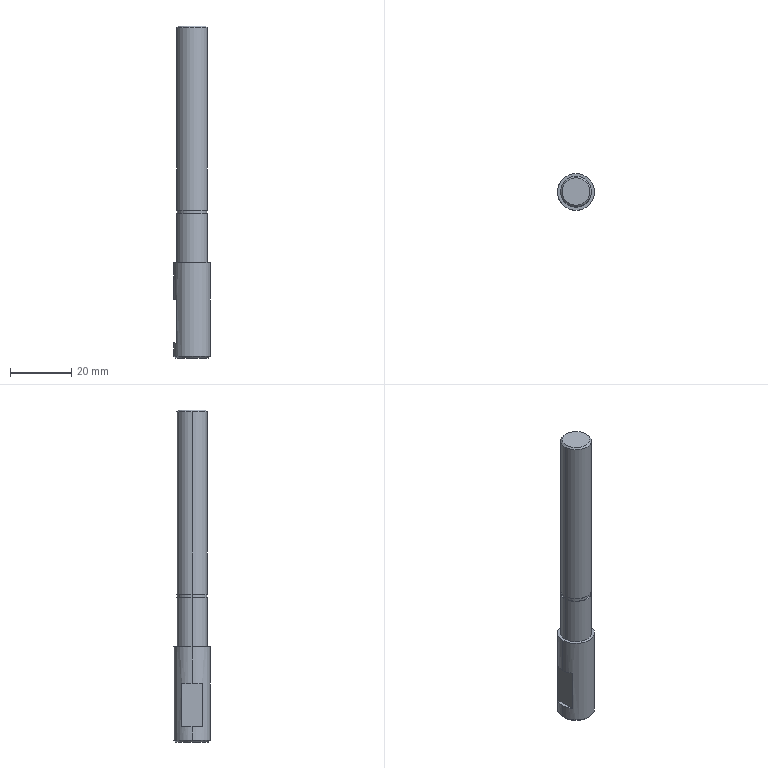Part | STEP file | PN_0097 linear shaft | 1 solid | 20 faces | box 12 x 12 x 108 mm | volume 9475 mm3 | cylinder 8 | plane 8 | cone 4 | commonest cylinder face diameters 10 x4 9.6 x2 12 x2
STEP:
#1=CARTESIAN_POINT('',(0.,0.,0.));
#2=DIRECTION('',(0.,0.,1.));
#3=DIRECTION('',(1.,0.,0.));
#4=AXIS2_PLACEMENT_3D('',#1,#2,#3);
#5=CARTESIAN_POINT('',(-5.5,0.,0.));
#6=VERTEX_POINT('',#5);
#7=CARTESIAN_POINT('',(5.5,0.,0.));
#8=VERTEX_POINT('',#7);
#9=CARTESIAN_POINT('',(0.,0.,0.));
#10=DIRECTION('',(0.,0.,-1.));
#11=DIRECTION('',(1.,0.,0.));
#12=AXIS2_PLACEMENT_3D('',#9,#10,#11);
#13=CIRCLE('',#12,5.5);
#14=CARTESIAN_POINT('',(0.,0.,0.5));
#15=DIRECTION('',(0.,0.,1.));
#16=DIRECTION('',(1.,0.,0.));
#17=AXIS2_PLACEMENT_3D('',#14,#15,#16);
#18=CONICAL_SURFACE('',#17,6.,0.7854);
#19=CARTESIAN_POINT('',(6.283,-0.5));
#20=DIRECTION('',(-1.,0.));
#21=VECTOR('',#20,1.);
#22=LINE('',#19,#21);
#23=(GEOMETRIC_REPRESENTATION_CONTEXT(2)PARAMETRIC_REPRESENTATION_CONTEXT()REPRESENTATION_CONTEXT('',''));
#24=DEFINITIONAL_REPRESENTATION('',(#22),#23);
#25=PCURVE('',#18,#24);
#26=CARTESIAN_POINT('',(0.,0.,0.));
#27=DIRECTION('',(0.,0.,1.));
#28=DIRECTION('',(1.,0.,0.));
#29=AXIS2_PLACEMENT_3D('',#26,#27,#28);
#30=PLANE('',#29);
#31=CARTESIAN_POINT('',(5.5,0.));
#32=CARTESIAN_POINT('',(5.5,-9.526));
#33=CARTESIAN_POINT('',(-2.75,-4.763));
#34=CARTESIAN_POINT('',(-11.,0.));
#35=CARTESIAN_POINT('',(-2.75,4.763));
#36=CARTESIAN_POINT('',(5.5,9.526));
#37=CARTESIAN_POINT('',(5.5,0.));
#38=(BOUNDED_CURVE()B_SPLINE_CURVE(2,(#31,#32,#33,#34,#35,#36,#37),.UNSPECIFIED.,.T.,.F.)B_SPLINE_CURVE_WITH_KNOTS((1,2,2,2,2,1),(-2.094,0.,2.094,4.189,6.283,8.378),.UNSPECIFIED.)CURVE()GEOMETRIC_REPRESENTATION_ITEM()RATIONAL_B_SPLINE_CURVE((1.,0.5,1.,0.5,1.,0.5,1.))REPRESENTATION_ITEM(''));
#39=(GEOMETRIC_REPRESENTATION_CONTEXT(2)PARAMETRIC_REPRESENTATION_CONTEXT()REPRESENTATION_CONTEXT('',''));
#40=DEFINITIONAL_REPRESENTATION('',(#38),#39);
#41=PCURVE('',#30,#40);
#42=SURFACE_CURVE('',#13,(#25,#41),.PCURVE_S1.);
#43=EDGE_CURVE('',#6,#8,#42,.T.);
#44=ORIENTED_EDGE('',*,*,#43,.F.);
#45=CARTESIAN_POINT('',(-6.,0.,0.5));
#46=VERTEX_POINT('',#45);
#47=CARTESIAN_POINT('',(-6.,0.,0.5));
#48=DIRECTION('',(-0.7071,0.,0.7071));
#49=VECTOR('',#48,1.);
#50=LINE('',#47,#49);
#51=CARTESIAN_POINT('',(3.142,0.));
#52=DIRECTION('',(0.,1.));
#53=VECTOR('',#52,1.);
#54=LINE('',#51,#53);
#55=(GEOMETRIC_REPRESENTATION_CONTEXT(2)PARAMETRIC_REPRESENTATION_CONTEXT()REPRESENTATION_CONTEXT('',''));
#56=DEFINITIONAL_REPRESENTATION('',(#54),#55);
#57=PCURVE('',#18,#56);
#58=CARTESIAN_POINT('',(0.,0.,0.5));
#59=DIRECTION('',(0.,0.,1.));
#60=DIRECTION('',(1.,0.,0.));
#61=AXIS2_PLACEMENT_3D('',#58,#59,#60);
#62=CONICAL_SURFACE('',#61,6.,0.7854);
#63=CARTESIAN_POINT('',(3.142,0.));
#64=DIRECTION('',(0.,1.));
#65=VECTOR('',#64,1.);
#66=LINE('',#63,#65);
#67=(GEOMETRIC_REPRESENTATION_CONTEXT(2)PARAMETRIC_REPRESENTATION_CONTEXT()REPRESENTATION_CONTEXT('',''));
#68=DEFINITIONAL_REPRESENTATION('',(#66),#67);
#69=PCURVE('',#62,#68);
#70=SURFACE_CURVE('',#50,(#57,#69),.PCURVE_S1.);
#71=EDGE_CURVE('',#6,#46,#70,.T.);
#72=ORIENTED_EDGE('',*,*,#71,.T.);
#73=CARTESIAN_POINT('',(6.,0.,0.5));
#74=VERTEX_POINT('',#73);
#75=CARTESIAN_POINT('',(0.,0.,0.5));
#76=DIRECTION('',(0.,0.,1.));
#77=DIRECTION('',(1.,0.,0.));
#78=AXIS2_PLACEMENT_3D('',#75,#76,#77);
#79=CIRCLE('',#78,6.);
#80=CARTESIAN_POINT('',(0.,0.));
#81=DIRECTION('',(1.,0.));
#82=VECTOR('',#81,1.);
#83=LINE('',#80,#82);
#84=(GEOMETRIC_REPRESENTATION_CONTEXT(2)PARAMETRIC_REPRESENTATION_CONTEXT()REPRESENTATION_CONTEXT('',''));
#85=DEFINITIONAL_REPRESENTATION('',(#83),#84);
#86=PCURVE('',#18,#85);
#87=CARTESIAN_POINT('',(0.,0.,31.));
#88=DIRECTION('',(0.,0.,-1.));
#89=DIRECTION('',(-1.,0.,0.));
#90=AXIS2_PLACEMENT_3D('',#87,#88,#89);
#91=CYLINDRICAL_SURFACE('',#90,6.);
#92=CARTESIAN_POINT('',(3.142,30.5));
#93=DIRECTION('',(-1.,0.));
#94=VECTOR('',#93,1.);
#95=LINE('',#92,#94);
#96=(GEOMETRIC_REPRESENTATION_CONTEXT(2)PARAMETRIC_REPRESENTATION_CONTEXT()REPRESENTATION_CONTEXT('',''));
#97=DEFINITIONAL_REPRESENTATION('',(#95),#96);
#98=PCURVE('',#91,#97);
#99=SURFACE_CURVE('',#79,(#86,#98),.PCURVE_S1.);
#100=EDGE_CURVE('',#74,#46,#99,.T.);
#101=ORIENTED_EDGE('',*,*,#100,.F.);
#102=CARTESIAN_POINT('',(6.,0.,0.5));
#103=DIRECTION('',(0.7071,0.,0.7071));
#104=VECTOR('',#103,1.);
#105=LINE('',#102,#104);
#106=CARTESIAN_POINT('',(0.,0.));
#107=DIRECTION('',(0.,1.));
#108=VECTOR('',#107,1.);
#109=LINE('',#106,#108);
#110=(GEOMETRIC_REPRESENTATION_CONTEXT(2)PARAMETRIC_REPRESENTATION_CONTEXT()REPRESENTATION_CONTEXT('',''));
#111=DEFINITIONAL_REPRESENTATION('',(#109),#110);
#112=PCURVE('',#18,#111);
#113=CARTESIAN_POINT('',(6.283,0.));
#114=DIRECTION('',(0.,1.));
#115=VECTOR('',#114,1.);
#116=LINE('',#113,#115);
#117=(GEOMETRIC_REPRESENTATION_CONTEXT(2)PARAMETRIC_REPRESENTATION_CONTEXT()REPRESENTATION_CONTEXT('',''));
#118=DEFINITIONAL_REPRESENTATION('',(#116),#117);
#119=PCURVE('',#62,#118);
#120=SURFACE_CURVE('',#105,(#112,#119),.PCURVE_S1.);
#121=EDGE_CURVE('',#8,#74,#120,.T.);
#122=ORIENTED_EDGE('',*,*,#121,.F.);
#123=EDGE_LOOP('',(#44,#72,#101,#122));
#124=FACE_BOUND('',#123,.T.);
#125=ADVANCED_FACE('',(#124),#18,.T.);
#126=CARTESIAN_POINT('',(4.5,0.,108.));
#127=VERTEX_POINT('',#126);
#128=CARTESIAN_POINT('',(-4.5,0.,108.));
#129=VERTEX_POINT('',#128);
#130=CARTESIAN_POINT('',(0.,0.,108.));
#131=DIRECTION('',(0.,0.,1.));
#132=DIRECTION('',(1.,0.,0.));
#133=AXIS2_PLACEMENT_3D('',#130,#131,#132);
#134=CIRCLE('',#133,4.5);
#135=CARTESIAN_POINT('',(0.,0.,108.));
#136=DIRECTION('',(0.,0.,-1.));
#137=DIRECTION('',(-1.,0.,0.));
#138=AXIS2_PLACEMENT_3D('',#135,#136,#137);
#139=CONICAL_SURFACE('',#138,4.5,0.7854);
#140=CARTESIAN_POINT('',(3.142,0.));
#141=DIRECTION('',(-1.,0.));
#142=VECTOR('',#141,1.);
#143=LINE('',#140,#142);
#144=(GEOMETRIC_REPRESENTATION_CONTEXT(2)PARAMETRIC_REPRESENTATION_CONTEXT()REPRESENTATION_CONTEXT('',''));
#145=DEFINITIONAL_REPRESENTATION('',(#143),#144);
#146=PCURVE('',#139,#145);
#147=CARTESIAN_POINT('',(0.,0.,108.));
#148=DIRECTION('',(0.,0.,1.));
#149=DIRECTION('',(1.,0.,0.));
#150=AXIS2_PLACEMENT_3D('',#147,#148,#149);
#151=PLANE('',#150);
#152=CARTESIAN_POINT('',(0.,0.));
#153=DIRECTION('',(1.,0.));
#154=AXIS2_PLACEMENT_2D('',#152,#153);
#155=CIRCLE('',#154,4.5);
#156=(GEOMETRIC_REPRESENTATION_CONTEXT(2)PARAMETRIC_REPRESENTATION_CONTEXT()REPRESENTATION_CONTEXT('',''));
#157=DEFINITIONAL_REPRESENTATION('',(#155),#156);
#158=PCURVE('',#151,#157);
#159=SURFACE_CURVE('',#134,(#146,#158),.PCURVE_S1.);
#160=EDGE_CURVE('',#127,#129,#159,.T.);
#161=ORIENTED_EDGE('',*,*,#160,.F.);
#162=CARTESIAN_POINT('',(5.,0.,107.5));
#163=VERTEX_POINT('',#162);
#164=CARTESIAN_POINT('',(4.5,0.,108.));
#165=DIRECTION('',(0.7071,0.,-0.7071));
#166=VECTOR('',#165,1.);
#167=LINE('',#164,#166);
#168=CARTESIAN_POINT('',(3.142,0.));
#169=DIRECTION('',(0.,1.));
#170=VECTOR('',#169,1.);
#171=LINE('',#168,#170);
#172=(GEOMETRIC_REPRESENTATION_CONTEXT(2)PARAMETRIC_REPRESENTATION_CONTEXT()REPRESENTATION_CONTEXT('',''));
#173=DEFINITIONAL_REPRESENTATION('',(#171),#172);
#174=PCURVE('',#139,#173);
#175=CARTESIAN_POINT('',(0.,0.,108.));
#176=DIRECTION('',(0.,0.,-1.));
#177=DIRECTION('',(-1.,0.,0.));
#178=AXIS2_PLACEMENT_3D('',#175,#176,#177);
#179=CONICAL_SURFACE('',#178,4.5,0.7854);
#180=CARTESIAN_POINT('',(3.142,0.));
#181=DIRECTION('',(0.,1.));
#182=VECTOR('',#181,1.);
#183=LINE('',#180,#182);
#184=(GEOMETRIC_REPRESENTATION_CONTEXT(2)PARAMETRIC_REPRESENTATION_CONTEXT()REPRESENTATION_CONTEXT('',''));
#185=DEFINITIONAL_REPRESENTATION('',(#183),#184);
#186=PCURVE('',#179,#185);
#187=SURFACE_CURVE('',#167,(#174,#186),.PCURVE_S1.);
#188=EDGE_CURVE('',#127,#163,#187,.T.);
#189=ORIENTED_EDGE('',*,*,#188,.T.);
#190=CARTESIAN_POINT('',(-5.,0.,107.5));
#191=VERTEX_POINT('',#190);
#192=CARTESIAN_POINT('',(0.,0.,107.5));
#193=DIRECTION('',(0.,0.,-1.));
#194=DIRECTION('',(1.,0.,0.));
#195=AXIS2_PLACEMENT_3D('',#192,#193,#194);
#196=CIRCLE('',#195,5.);
#197=CARTESIAN_POINT('',(-3.142,0.5));
#198=DIRECTION('',(1.,0.));
#199=VECTOR('',#198,1.);
#200=LINE('',#197,#199);
#201=(GEOMETRIC_REPRESENTATION_CONTEXT(2)PARAMETRIC_REPRESENTATION_CONTEXT()REPRESENTATION_CONTEXT('',''));
#202=DEFINITIONAL_REPRESENTATION('',(#200),#201);
#203=PCURVE('',#139,#202);
#204=CARTESIAN_POINT('',(0.,0.,108.));
#205=DIRECTION('',(0.,0.,-1.));
#206=DIRECTION('',(-1.,0.,0.));
#207=AXIS2_PLACEMENT_3D('',#204,#205,#206);
#208=CYLINDRICAL_SURFACE('',#207,5.);
#209=CARTESIAN_POINT('',(-3.142,0.5));
#210=DIRECTION('',(1.,0.));
#211=VECTOR('',#210,1.);
#212=LINE('',#209,#211);
#213=(GEOMETRIC_REPRESENTATION_CONTEXT(2)PARAMETRIC_REPRESENTATION_CONTEXT()REPRESENTATION_CONTEXT('',''));
#214=DEFINITIONAL_REPRESENTATION('',(#212),#213);
#215=PCURVE('',#208,#214);
#216=SURFACE_CURVE('',#196,(#203,#215),.PCURVE_S1.);
#217=EDGE_CURVE('',#191,#163,#216,.T.);
#218=ORIENTED_EDGE('',*,*,#217,.F.);
#219=CARTESIAN_POINT('',(-4.5,0.,108.));
#220=DIRECTION('',(-0.7071,0.,-0.7071));
#221=VECTOR('',#220,1.);
#222=LINE('',#219,#221);
#223=CARTESIAN_POINT('',(0.,0.));
#224=DIRECTION('',(0.,1.));
#225=VECTOR('',#224,1.);
#226=LINE('',#223,#225);
#227=(GEOMETRIC_REPRESENTATION_CONTEXT(2)PARAMETRIC_REPRESENTATION_CONTEXT()REPRESENTATION_CONTEXT('',''));
#228=DEFINITIONAL_REPRESENTATION('',(#226),#227);
#229=PCURVE('',#139,#228);
#230=CARTESIAN_POINT('',(6.283,0.));
#231=DIRECTION('',(0.,1.));
#232=VECTOR('',#231,1.);
#233=LINE('',#230,#232);
#234=(GEOMETRIC_REPRESENTATION_CONTEXT(2)PARAMETRIC_REPRESENTATION_CONTEXT()REPRESENTATION_CONTEXT('',''));
#235=DEFINITIONAL_REPRESENTATION('',(#233),#234);
#236=PCURVE('',#179,#235);
#237=SURFACE_CURVE('',#222,(#229,#236),.PCURVE_S1.);
#238=EDGE_CURVE('',#129,#191,#237,.T.);
#239=ORIENTED_EDGE('',*,*,#238,.F.);
#240=EDGE_LOOP('',(#161,#189,#218,#239));
#241=FACE_BOUND('',#240,.T.);
#242=ADVANCED_FACE('',(#241),#139,.T.);
#243=ORIENTED_EDGE('',*,*,#217,.T.);
#244=CARTESIAN_POINT('',(5.,0.,48.1));
#245=VERTEX_POINT('',#244);
#246=CARTESIAN_POINT('',(5.,0.,108.));
#247=DIRECTION('',(0.,0.,-1.));
#248=VECTOR('',#247,1.);
#249=LINE('',#246,#248);
#250=CARTESIAN_POINT('',(3.142,0.));
#251=DIRECTION('',(0.,1.));
#252=VECTOR('',#251,1.);
#253=LINE('',#250,#252);
#254=(GEOMETRIC_REPRESENTATION_CONTEXT(2)PARAMETRIC_REPRESENTATION_CONTEXT()REPRESENTATION_CONTEXT('',''));
#255=DEFINITIONAL_REPRESENTATION('',(#253),#254);
#256=PCURVE('',#208,#255);
#257=CARTESIAN_POINT('',(0.,0.,108.));
#258=DIRECTION('',(0.,0.,-1.));
#259=DIRECTION('',(-1.,0.,0.));
#260=AXIS2_PLACEMENT_3D('',#257,#258,#259);
#261=CYLINDRICAL_SURFACE('',#260,5.);
#262=CARTESIAN_POINT('',(3.142,0.));
#263=DIRECTION('',(0.,1.));
#264=VECTOR('',#263,1.);
#265=LINE('',#262,#264);
#266=(GEOMETRIC_REPRESENTATION_CONTEXT(2)PARAMETRIC_REPRESENTATION_CONTEXT()REPRESENTATION_CONTEXT('',''));
#267=DEFINITIONAL_REPRESENTATION('',(#265),#266);
#268=PCURVE('',#261,#267);
#269=SURFACE_CURVE('',#249,(#256,#268),.PCURVE_S1.);
#270=EDGE_CURVE('',#163,#245,#269,.T.);
#271=ORIENTED_EDGE('',*,*,#270,.T.);
#272=CARTESIAN_POINT('',(-5.,0.,48.1));
#273=VERTEX_POINT('',#272);
#274=CARTESIAN_POINT('',(0.,0.,48.1));
#275=DIRECTION('',(0.,0.,1.));
#276=DIRECTION('',(1.,0.,0.));
#277=AXIS2_PLACEMENT_3D('',#274,#275,#276);
#278=CIRCLE('',#277,5.);
#279=CARTESIAN_POINT('',(3.142,59.9));
#280=DIRECTION('',(-1.,0.));
#281=VECTOR('',#280,1.);
#282=LINE('',#279,#281);
#283=(GEOMETRIC_REPRESENTATION_CONTEXT(2)PARAMETRIC_REPRESENTATION_CONTEXT()REPRESENTATION_CONTEXT('',''));
#284=DEFINITIONAL_REPRESENTATION('',(#282),#283);
#285=PCURVE('',#208,#284);
#286=CARTESIAN_POINT('',(0.,0.,48.1));
#287=DIRECTION('',(0.,0.,1.));
#288=DIRECTION('',(1.,0.,0.));
#289=AXIS2_PLACEMENT_3D('',#286,#287,#288);
#290=PLANE('',#289);
#291=CARTESIAN_POINT('',(0.,0.));
#292=DIRECTION('',(1.,0.));
#293=AXIS2_PLACEMENT_2D('',#291,#292);
#294=CIRCLE('',#293,5.);
#295=(GEOMETRIC_REPRESENTATION_CONTEXT(2)PARAMETRIC_REPRESENTATION_CONTEXT()REPRESENTATION_CONTEXT('',''));
#296=DEFINITIONAL_REPRESENTATION('',(#294),#295);
#297=PCURVE('',#290,#296);
#298=SURFACE_CURVE('',#278,(#285,#297),.PCURVE_S1.);
#299=EDGE_CURVE('',#245,#273,#298,.T.);
#300=ORIENTED_EDGE('',*,*,#299,.T.);
#301=CARTESIAN_POINT('',(-5.,0.,108.));
#302=DIRECTION('',(0.,0.,-1.));
#303=VECTOR('',#302,1.);
#304=LINE('',#301,#303);
#305=CARTESIAN_POINT('',(0.,0.));
#306=DIRECTION('',(0.,1.));
#307=VECTOR('',#306,1.);
#308=LINE('',#305,#307);
#309=(GEOMETRIC_REPRESENTATION_CONTEXT(2)PARAMETRIC_REPRESENTATION_CONTEXT()REPRESENTATION_CONTEXT('',''));
#310=DEFINITIONAL_REPRESENTATION('',(#308),#309);
#311=PCURVE('',#208,#310);
#312=CARTESIAN_POINT('',(6.283,0.));
#313=DIRECTION('',(0.,1.));
#314=VECTOR('',#313,1.);
#315=LINE('',#312,#314);
#316=(GEOMETRIC_REPRESENTATION_CONTEXT(2)PARAMETRIC_REPRESENTATION_CONTEXT()REPRESENTATION_CONTEXT('',''));
#317=DEFINITIONAL_REPRESENTATION('',(#315),#316);
#318=PCURVE('',#261,#317);
#319=SURFACE_CURVE('',#304,(#311,#318),.PCURVE_S1.);
#320=EDGE_CURVE('',#191,#273,#319,.T.);
#321=ORIENTED_EDGE('',*,*,#320,.F.);
#322=EDGE_LOOP('',(#243,#271,#300,#321));
#323=FACE_BOUND('',#322,.T.);
#324=ADVANCED_FACE('',(#323),#208,.T.);
#325=CARTESIAN_POINT('',(4.8,0.,48.1));
#326=VERTEX_POINT('',#325);
#327=CARTESIAN_POINT('',(-4.8,0.,48.1));
#328=VERTEX_POINT('',#327);
#329=CARTESIAN_POINT('',(0.,0.,48.1));
#330=DIRECTION('',(0.,0.,1.));
#331=DIRECTION('',(1.,0.,0.));
#332=AXIS2_PLACEMENT_3D('',#329,#330,#331);
#333=CIRCLE('',#332,4.8);
#334=CARTESIAN_POINT('',(0.,0.,48.1));
#335=DIRECTION('',(0.,0.,-1.));
#336=DIRECTION('',(-1.,0.,0.));
#337=AXIS2_PLACEMENT_3D('',#334,#335,#336);
#338=CYLINDRICAL_SURFACE('',#337,4.8);
#339=CARTESIAN_POINT('',(3.142,0.));
#340=DIRECTION('',(-1.,0.));
#341=VECTOR('',#340,1.);
#342=LINE('',#339,#341);
#343=(GEOMETRIC_REPRESENTATION_CONTEXT(2)PARAMETRIC_REPRESENTATION_CONTEXT()REPRESENTATION_CONTEXT('',''));
#344=DEFINITIONAL_REPRESENTATION('',(#342),#343);
#345=PCURVE('',#338,#344);
#346=CARTESIAN_POINT('',(0.,0.));
#347=DIRECTION('',(1.,0.));
#348=AXIS2_PLACEMENT_2D('',#346,#347);
#349=CIRCLE('',#348,4.8);
#350=(GEOMETRIC_REPRESENTATION_CONTEXT(2)PARAMETRIC_REPRESENTATION_CONTEXT()REPRESENTATION_CONTEXT('',''));
#351=DEFINITIONAL_REPRESENTATION('',(#349),#350);
#352=PCURVE('',#290,#351);
#353=SURFACE_CURVE('',#333,(#345,#352),.PCURVE_S1.);
#354=EDGE_CURVE('',#326,#328,#353,.T.);
#355=ORIENTED_EDGE('',*,*,#354,.F.);
#356=CARTESIAN_POINT('',(4.8,0.,47.));
#357=VERTEX_POINT('',#356);
#358=CARTESIAN_POINT('',(4.8,0.,48.1));
#359=DIRECTION('',(0.,0.,-1.));
#360=VECTOR('',#359,1.);
#361=LINE('',#358,#360);
#362=CARTESIAN_POINT('',(3.142,0.));
#363=DIRECTION('',(0.,1.));
#364=VECTOR('',#363,1.);
#365=LINE('',#362,#364);
#366=(GEOMETRIC_REPRESENTATION_CONTEXT(2)PARAMETRIC_REPRESENTATION_CONTEXT()REPRESENTATION_CONTEXT('',''));
#367=DEFINITIONAL_REPRESENTATION('',(#365),#366);
#368=PCURVE('',#338,#367);
#369=CARTESIAN_POINT('',(0.,0.,48.1));
#370=DIRECTION('',(0.,0.,-1.));
#371=DIRECTION('',(-1.,0.,0.));
#372=AXIS2_PLACEMENT_3D('',#369,#370,#371);
#373=CYLINDRICAL_SURFACE('',#372,4.8);
#374=CARTESIAN_POINT('',(3.142,0.));
#375=DIRECTION('',(0.,1.));
#376=VECTOR('',#375,1.);
#377=LINE('',#374,#376);
#378=(GEOMETRIC_REPRESENTATION_CONTEXT(2)PARAMETRIC_REPRESENTATION_CONTEXT()REPRESENTATION_CONTEXT('',''));
#379=DEFINITIONAL_REPRESENTATION('',(#377),#378);
#380=PCURVE('',#373,#379);
#381=SURFACE_CURVE('',#361,(#368,#380),.PCURVE_S1.);
#382=EDGE_CURVE('',#326,#357,#381,.T.);
#383=ORIENTED_EDGE('',*,*,#382,.T.);
#384=CARTESIAN_POINT('',(-4.8,0.,47.));
#385=VERTEX_POINT('',#384);
#386=CARTESIAN_POINT('',(0.,0.,47.));
#387=DIRECTION('',(0.,0.,1.));
#388=DIRECTION('',(1.,0.,0.));
#389=AXIS2_PLACEMENT_3D('',#386,#387,#388);
#390=CIRCLE('',#389,4.8);
#391=CARTESIAN_POINT('',(3.142,1.1));
#392=DIRECTION('',(-1.,0.));
#393=VECTOR('',#392,1.);
#394=LINE('',#391,#393);
#395=(GEOMETRIC_REPRESENTATION_CONTEXT(2)PARAMETRIC_REPRESENTATION_CONTEXT()REPRESENTATION_CONTEXT('',''));
#396=DEFINITIONAL_REPRESENTATION('',(#394),#395);
#397=PCURVE('',#338,#396);
#398=CARTESIAN_POINT('',(0.,0.,47.));
#399=DIRECTION('',(0.,0.,1.));
#400=DIRECTION('',(1.,0.,0.));
#401=AXIS2_PLACEMENT_3D('',#398,#399,#400);
#402=PLANE('',#401);
#403=CARTESIAN_POINT('',(0.,0.));
#404=DIRECTION('',(1.,0.));
#405=AXIS2_PLACEMENT_2D('',#403,#404);
#406=CIRCLE('',#405,4.8);
#407=(GEOMETRIC_REPRESENTATION_CONTEXT(2)PARAMETRIC_REPRESENTATION_CONTEXT()REPRESENTATION_CONTEXT('',''));
#408=DEFINITIONAL_REPRESENTATION('',(#406),#407);
#409=PCURVE('',#402,#408);
#410=SURFACE_CURVE('',#390,(#397,#409),.PCURVE_S1.);
#411=EDGE_CURVE('',#357,#385,#410,.T.);
#412=ORIENTED_EDGE('',*,*,#411,.T.);
#413=CARTESIAN_POINT('',(-4.8,0.,48.1));
#414=DIRECTION('',(0.,0.,-1.));
#415=VECTOR('',#414,1.);
#416=LINE('',#413,#415);
#417=CARTESIAN_POINT('',(0.,0.));
#418=DIRECTION('',(0.,1.));
#419=VECTOR('',#418,1.);
#420=LINE('',#417,#419);
#421=(GEOMETRIC_REPRESENTATION_CONTEXT(2)PARAMETRIC_REPRESENTATION_CONTEXT()REPRESENTATION_CONTEXT('',''));
#422=DEFINITIONAL_REPRESENTATION('',(#420),#421);
#423=PCURVE('',#338,#422);
#424=CARTESIAN_POINT('',(6.283,0.));
#425=DIRECTION('',(0.,1.));
#426=VECTOR('',#425,1.);
#427=LINE('',#424,#426);
#428=(GEOMETRIC_REPRESENTATION_CONTEXT(2)PARAMETRIC_REPRESENTATION_CONTEXT()REPRESENTATION_CONTEXT('',''));
#429=DEFINITIONAL_REPRESENTATION('',(#427),#428);
#430=PCURVE('',#373,#429);
#431=SURFACE_CURVE('',#416,(#423,#430),.PCURVE_S1.);
#432=EDGE_CURVE('',#328,#385,#431,.T.);
#433=ORIENTED_EDGE('',*,*,#432,.F.);
#434=EDGE_LOOP('',(#355,#383,#412,#433));
#435=FACE_BOUND('',#434,.T.);
#436=ADVANCED_FACE('',(#435),#338,.T.);
#437=CARTESIAN_POINT('',(5.,0.,47.));
#438=VERTEX_POINT('',#437);
#439=CARTESIAN_POINT('',(-5.,0.,47.));
#440=VERTEX_POINT('',#439);
#441=CARTESIAN_POINT('',(0.,0.,47.));
#442=DIRECTION('',(0.,0.,1.));
#443=DIRECTION('',(1.,0.,0.));
#444=AXIS2_PLACEMENT_3D('',#441,#442,#443);
#445=CIRCLE('',#444,5.);
#446=CARTESIAN_POINT('',(0.,0.,47.));
#447=DIRECTION('',(0.,0.,-1.));
#448=DIRECTION('',(-1.,0.,0.));
#449=AXIS2_PLACEMENT_3D('',#446,#447,#448);
#450=CYLINDRICAL_SURFACE('',#449,5.);
#451=CARTESIAN_POINT('',(3.142,0.));
#452=DIRECTION('',(-1.,0.));
#453=VECTOR('',#452,1.);
#454=LINE('',#451,#453);
#455=(GEOMETRIC_REPRESENTATION_CONTEXT(2)PARAMETRIC_REPRESENTATION_CONTEXT()REPRESENTATION_CONTEXT('',''));
#456=DEFINITIONAL_REPRESENTATION('',(#454),#455);
#457=PCURVE('',#450,#456);
#458=CARTESIAN_POINT('',(0.,0.));
#459=DIRECTION('',(1.,0.));
#460=AXIS2_PLACEMENT_2D('',#458,#459);
#461=CIRCLE('',#460,5.);
#462=(GEOMETRIC_REPRESENTATION_CONTEXT(2)PARAMETRIC_REPRESENTATION_CONTEXT()REPRESENTATION_CONTEXT('',''));
#463=DEFINITIONAL_REPRESENTATION('',(#461),#462);
#464=PCURVE('',#402,#463);
#465=SURFACE_CURVE('',#445,(#457,#464),.PCURVE_S1.);
#466=EDGE_CURVE('',#438,#440,#465,.T.);
#467=ORIENTED_EDGE('',*,*,#466,.F.);
#468=CARTESIAN_POINT('',(5.,0.,31.));
#469=VERTEX_POINT('',#468);
#470=CARTESIAN_POINT('',(5.,0.,47.));
#471=DIRECTION('',(0.,0.,-1.));
#472=VECTOR('',#471,1.);
#473=LINE('',#470,#472);
#474=CARTESIAN_POINT('',(3.142,0.));
#475=DIRECTION('',(0.,1.));
#476=VECTOR('',#475,1.);
#477=LINE('',#474,#476);
#478=(GEOMETRIC_REPRESENTATION_CONTEXT(2)PARAMETRIC_REPRESENTATION_CONTEXT()REPRESENTATION_CONTEXT('',''));
#479=DEFINITIONAL_REPRESENTATION('',(#477),#478);
#480=PCURVE('',#450,#479);
#481=CARTESIAN_POINT('',(0.,0.,47.));
#482=DIRECTION('',(0.,0.,-1.));
#483=DIRECTION('',(-1.,0.,0.));
#484=AXIS2_PLACEMENT_3D('',#481,#482,#483);
#485=CYLINDRICAL_SURFACE('',#484,5.);
#486=CARTESIAN_POINT('',(3.142,0.));
#487=DIRECTION('',(0.,1.));
#488=VECTOR('',#487,1.);
#489=LINE('',#486,#488);
#490=(GEOMETRIC_REPRESENTATION_CONTEXT(2)PARAMETRIC_REPRESENTATION_CONTEXT()REPRESENTATION_CONTEXT('',''));
#491=DEFINITIONAL_REPRESENTATION('',(#489),#490);
#492=PCURVE('',#485,#491);
#493=SURFACE_CURVE('',#473,(#480,#492),.PCURVE_S1.);
#494=EDGE_CURVE('',#438,#469,#493,.T.);
#495=ORIENTED_EDGE('',*,*,#494,.T.);
#496=CARTESIAN_POINT('',(-5.,0.,31.));
#497=VERTEX_POINT('',#496);
#498=CARTESIAN_POINT('',(0.,0.,31.));
#499=DIRECTION('',(0.,0.,1.));
#500=DIRECTION('',(1.,0.,0.));
#501=AXIS2_PLACEMENT_3D('',#498,#499,#500);
#502=CIRCLE('',#501,5.);
#503=CARTESIAN_POINT('',(3.142,16.));
#504=DIRECTION('',(-1.,0.));
#505=VECTOR('',#504,1.);
#506=LINE('',#503,#505);
#507=(GEOMETRIC_REPRESENTATION_CONTEXT(2)PARAMETRIC_REPRESENTATION_CONTEXT()REPRESENTATION_CONTEXT('',''));
#508=DEFINITIONAL_REPRESENTATION('',(#506),#507);
#509=PCURVE('',#450,#508);
#510=CARTESIAN_POINT('',(0.,0.,31.));
#511=DIRECTION('',(0.,0.,1.));
#512=DIRECTION('',(1.,0.,0.));
#513=AXIS2_PLACEMENT_3D('',#510,#511,#512);
#514=PLANE('',#513);
#515=CARTESIAN_POINT('',(0.,0.));
#516=DIRECTION('',(1.,0.));
#517=AXIS2_PLACEMENT_2D('',#515,#516);
#518=CIRCLE('',#517,5.);
#519=(GEOMETRIC_REPRESENTATION_CONTEXT(2)PARAMETRIC_REPRESENTATION_CONTEXT()REPRESENTATION_CONTEXT('',''));
#520=DEFINITIONAL_REPRESENTATION('',(#518),#519);
#521=PCURVE('',#514,#520);
#522=SURFACE_CURVE('',#502,(#509,#521),.PCURVE_S1.);
#523=EDGE_CURVE('',#469,#497,#522,.T.);
#524=ORIENTED_EDGE('',*,*,#523,.T.);
#525=CARTESIAN_POINT('',(-5.,0.,47.));
#526=DIRECTION('',(0.,0.,-1.));
#527=VECTOR('',#526,1.);
#528=LINE('',#525,#527);
#529=CARTESIAN_POINT('',(0.,0.));
#530=DIRECTION('',(0.,1.));
#531=VECTOR('',#530,1.);
#532=LINE('',#529,#531);
#533=(GEOMETRIC_REPRESENTATION_CONTEXT(2)PARAMETRIC_REPRESENTATION_CONTEXT()REPRESENTATION_CONTEXT('',''));
#534=DEFINITIONAL_REPRESENTATION('',(#532),#533);
#535=PCURVE('',#450,#534);
#536=CARTESIAN_POINT('',(6.283,0.));
#537=DIRECTION('',(0.,1.));
#538=VECTOR('',#537,1.);
#539=LINE('',#536,#538);
#540=(GEOMETRIC_REPRESENTATION_CONTEXT(2)PARAMETRIC_REPRESENTATION_CONTEXT()REPRESENTATION_CONTEXT('',''));
#541=DEFINITIONAL_REPRESENTATION('',(#539),#540);
#542=PCURVE('',#485,#541);
#543=SURFACE_CURVE('',#528,(#535,#542),.PCURVE_S1.);
#544=EDGE_CURVE('',#440,#497,#543,.T.);
#545=ORIENTED_EDGE('',*,*,#544,.F.);
#546=EDGE_LOOP('',(#467,#495,#524,#545));
#547=FACE_BOUND('',#546,.T.);
#548=ADVANCED_FACE('',(#547),#450,.T.);
#549=CARTESIAN_POINT('',(6.,0.,31.));
#550=VERTEX_POINT('',#549);
#551=CARTESIAN_POINT('',(-6.,0.,31.));
#552=VERTEX_POINT('',#551);
#553=CARTESIAN_POINT('',(0.,0.,31.));
#554=DIRECTION('',(0.,0.,1.));
#555=DIRECTION('',(1.,0.,0.));
#556=AXIS2_PLACEMENT_3D('',#553,#554,#555);
#557=CIRCLE('',#556,6.);
#558=CARTESIAN_POINT('',(3.142,0.));
#559=DIRECTION('',(-1.,0.));
#560=VECTOR('',#559,1.);
#561=LINE('',#558,#560);
#562=(GEOMETRIC_REPRESENTATION_CONTEXT(2)PARAMETRIC_REPRESENTATION_CONTEXT()REPRESENTATION_CONTEXT('',''));
#563=DEFINITIONAL_REPRESENTATION('',(#561),#562);
#564=PCURVE('',#91,#563);
#565=CARTESIAN_POINT('',(0.,0.));
#566=DIRECTION('',(1.,0.));
#567=AXIS2_PLACEMENT_2D('',#565,#566);
#568=CIRCLE('',#567,6.);
#569=(GEOMETRIC_REPRESENTATION_CONTEXT(2)PARAMETRIC_REPRESENTATION_CONTEXT()REPRESENTATION_CONTEXT('',''));
#570=DEFINITIONAL_REPRESENTATION('',(#568),#569);
#571=PCURVE('',#514,#570);
#572=SURFACE_CURVE('',#557,(#564,#571),.PCURVE_S1.);
#573=EDGE_CURVE('',#550,#552,#572,.T.);
#574=ORIENTED_EDGE('',*,*,#573,.F.);
#575=CARTESIAN_POINT('',(6.,0.,31.));
#576=DIRECTION('',(0.,0.,-1.));
#577=VECTOR('',#576,1.);
#578=LINE('',#575,#577);
#579=CARTESIAN_POINT('',(3.142,0.));
#580=DIRECTION('',(0.,1.));
#581=VECTOR('',#580,1.);
#582=LINE('',#579,#581);
#583=(GEOMETRIC_REPRESENTATION_CONTEXT(2)PARAMETRIC_REPRESENTATION_CONTEXT()REPRESENTATION_CONTEXT('',''));
#584=DEFINITIONAL_REPRESENTATION('',(#582),#583);
#585=PCURVE('',#91,#584);
#586=CARTESIAN_POINT('',(0.,0.,31.));
#587=DIRECTION('',(0.,0.,-1.));
#588=DIRECTION('',(-1.,0.,0.));
#589=AXIS2_PLACEMENT_3D('',#586,#587,#588);
#590=CYLINDRICAL_SURFACE('',#589,6.);
#591=CARTESIAN_POINT('',(3.142,0.));
#592=DIRECTION('',(0.,1.));
#593=VECTOR('',#592,1.);
#594=LINE('',#591,#593);
#595=(GEOMETRIC_REPRESENTATION_CONTEXT(2)PARAMETRIC_REPRESENTATION_CONTEXT()REPRESENTATION_CONTEXT('',''));
#596=DEFINITIONAL_REPRESENTATION('',(#594),#595);
#597=PCURVE('',#590,#596);
#598=SURFACE_CURVE('',#578,(#585,#597),.PCURVE_S1.);
#599=EDGE_CURVE('',#550,#74,#598,.T.);
#600=ORIENTED_EDGE('',*,*,#599,.T.);
#601=ORIENTED_EDGE('',*,*,#100,.T.);
#602=CARTESIAN_POINT('',(-6.,0.,5.));
#603=VERTEX_POINT('',#602);
#604=CARTESIAN_POINT('',(-6.,0.,31.));
#605=DIRECTION('',(0.,0.,-1.));
#606=VECTOR('',#605,1.);
#607=LINE('',#604,#606);
#608=CARTESIAN_POINT('',(0.,0.));
#609=DIRECTION('',(0.,1.));
#610=VECTOR('',#609,1.);
#611=LINE('',#608,#610);
#612=(GEOMETRIC_REPRESENTATION_CONTEXT(2)PARAMETRIC_REPRESENTATION_CONTEXT()REPRESENTATION_CONTEXT('',''));
#613=DEFINITIONAL_REPRESENTATION('',(#611),#612);
#614=PCURVE('',#91,#613);
#615=CARTESIAN_POINT('',(6.283,0.));
#616=DIRECTION('',(0.,1.));
#617=VECTOR('',#616,1.);
#618=LINE('',#615,#617);
#619=(GEOMETRIC_REPRESENTATION_CONTEXT(2)PARAMETRIC_REPRESENTATION_CONTEXT()REPRESENTATION_CONTEXT('',''));
#620=DEFINITIONAL_REPRESENTATION('',(#618),#619);
#621=PCURVE('',#590,#620);
#622=SURFACE_CURVE('',#607,(#614,#621),.PCURVE_S1.);
#623=EDGE_CURVE('',#603,#46,#622,.T.);
#624=ORIENTED_EDGE('',*,*,#623,.F.);
#625=CARTESIAN_POINT('',(-5.,3.317,5.));
#626=VERTEX_POINT('',#625);
#627=CARTESIAN_POINT('',(0.,0.,5.));
#628=DIRECTION('',(0.,0.,1.));
#629=DIRECTION('',(1.,0.,0.));
#630=AXIS2_PLACEMENT_3D('',#627,#628,#629);
#631=CIRCLE('',#630,6.);
#632=CARTESIAN_POINT('',(3.142,26.));
#633=DIRECTION('',(-1.,0.));
#634=VECTOR('',#633,1.);
#635=LINE('',#632,#634);
#636=(GEOMETRIC_REPRESENTATION_CONTEXT(2)PARAMETRIC_REPRESENTATION_CONTEXT()REPRESENTATION_CONTEXT('',''));
#637=DEFINITIONAL_REPRESENTATION('',(#635),#636);
#638=PCURVE('',#91,#637);
#639=CARTESIAN_POINT('',(-10.784,10.,5.));
#640=DIRECTION('',(0.,0.,1.));
#641=DIRECTION('',(1.,0.,0.));
#642=AXIS2_PLACEMENT_3D('',#639,#640,#641);
#643=PLANE('',#642);
#644=CARTESIAN_POINT('',(10.784,-10.));
#645=DIRECTION('',(1.,0.));
#646=AXIS2_PLACEMENT_2D('',#644,#645);
#647=CIRCLE('',#646,6.);
#648=(GEOMETRIC_REPRESENTATION_CONTEXT(2)PARAMETRIC_REPRESENTATION_CONTEXT()REPRESENTATION_CONTEXT('',''));
#649=DEFINITIONAL_REPRESENTATION('',(#647),#648);
#650=PCURVE('',#643,#649);
#651=SURFACE_CURVE('',#631,(#638,#650),.PCURVE_S1.);
#652=EDGE_CURVE('',#626,#603,#651,.T.);
#653=ORIENTED_EDGE('',*,*,#652,.F.);
#654=CARTESIAN_POINT('',(-5.,3.317,19.));
#655=VERTEX_POINT('',#654);
#656=CARTESIAN_POINT('',(-5.,3.317,31.));
#657=DIRECTION('',(0.,0.,-1.));
#658=VECTOR('',#657,1.);
#659=LINE('',#656,#658);
#660=CARTESIAN_POINT('',(0.5857,0.));
#661=DIRECTION('',(0.,1.));
#662=VECTOR('',#661,1.);
#663=LINE('',#660,#662);
#664=(GEOMETRIC_REPRESENTATION_CONTEXT(2)PARAMETRIC_REPRESENTATION_CONTEXT()REPRESENTATION_CONTEXT('',''));
#665=DEFINITIONAL_REPRESENTATION('',(#663),#664);
#666=PCURVE('',#91,#665);
#667=CARTESIAN_POINT('',(-5.,10.,5.));
#668=DIRECTION('',(-1.,0.,0.));
#669=DIRECTION('',(0.,0.,1.));
#670=AXIS2_PLACEMENT_3D('',#667,#668,#669);
#671=PLANE('',#670);
#672=CARTESIAN_POINT('',(26.,-6.683));
#673=DIRECTION('',(-1.,0.));
#674=VECTOR('',#673,1.);
#675=LINE('',#672,#674);
#676=(GEOMETRIC_REPRESENTATION_CONTEXT(2)PARAMETRIC_REPRESENTATION_CONTEXT()REPRESENTATION_CONTEXT('',''));
#677=DEFINITIONAL_REPRESENTATION('',(#675),#676);
#678=PCURVE('',#671,#677);
#679=SURFACE_CURVE('',#659,(#666,#678),.PCURVE_S1.);
#680=EDGE_CURVE('',#655,#626,#679,.T.);
#681=ORIENTED_EDGE('',*,*,#680,.F.);
#682=CARTESIAN_POINT('',(-6.,0.,19.));
#683=VERTEX_POINT('',#682);
#684=CARTESIAN_POINT('',(0.,0.,19.));
#685=DIRECTION('',(0.,0.,-1.));
#686=DIRECTION('',(-1.,0.,0.));
#687=AXIS2_PLACEMENT_3D('',#684,#685,#686);
#688=CIRCLE('',#687,6.);
#689=CARTESIAN_POINT('',(0.,12.));
#690=DIRECTION('',(1.,0.));
#691=VECTOR('',#690,1.);
#692=LINE('',#689,#691);
#693=(GEOMETRIC_REPRESENTATION_CONTEXT(2)PARAMETRIC_REPRESENTATION_CONTEXT()REPRESENTATION_CONTEXT('',''));
#694=DEFINITIONAL_REPRESENTATION('',(#692),#693);
#695=PCURVE('',#91,#694);
#696=CARTESIAN_POINT('',(-10.784,10.,19.));
#697=DIRECTION('',(0.,0.,-1.));
#698=DIRECTION('',(-1.,0.,0.));
#699=AXIS2_PLACEMENT_3D('',#696,#697,#698);
#700=PLANE('',#699);
#701=CARTESIAN_POINT('',(-10.784,-10.));
#702=DIRECTION('',(1.,0.));
#703=AXIS2_PLACEMENT_2D('',#701,#702);
#704=CIRCLE('',#703,6.);
#705=(GEOMETRIC_REPRESENTATION_CONTEXT(2)PARAMETRIC_REPRESENTATION_CONTEXT()REPRESENTATION_CONTEXT('',''));
#706=DEFINITIONAL_REPRESENTATION('',(#704),#705);
#707=PCURVE('',#700,#706);
#708=SURFACE_CURVE('',#688,(#695,#707),.PCURVE_S1.);
#709=EDGE_CURVE('',#683,#655,#708,.T.);
#710=ORIENTED_EDGE('',*,*,#709,.F.);
#711=CARTESIAN_POINT('',(-6.,0.,31.));
#712=DIRECTION('',(0.,0.,-1.));
#713=VECTOR('',#712,1.);
#714=LINE('',#711,#713);
#715=CARTESIAN_POINT('',(0.,0.));
#716=DIRECTION('',(0.,1.));
#717=VECTOR('',#716,1.);
#718=LINE('',#715,#717);
#719=(GEOMETRIC_REPRESENTATION_CONTEXT(2)PARAMETRIC_REPRESENTATION_CONTEXT()REPRESENTATION_CONTEXT('',''));
#720=DEFINITIONAL_REPRESENTATION('',(#718),#719);
#721=PCURVE('',#91,#720);
#722=CARTESIAN_POINT('',(6.283,0.));
#723=DIRECTION('',(0.,1.));
#724=VECTOR('',#723,1.);
#725=LINE('',#722,#724);
#726=(GEOMETRIC_REPRESENTATION_CONTEXT(2)PARAMETRIC_REPRESENTATION_CONTEXT()REPRESENTATION_CONTEXT('',''));
#727=DEFINITIONAL_REPRESENTATION('',(#725),#726);
#728=PCURVE('',#590,#727);
#729=SURFACE_CURVE('',#714,(#721,#728),.PCURVE_S1.);
#730=EDGE_CURVE('',#552,#683,#729,.T.);
#731=ORIENTED_EDGE('',*,*,#730,.F.);
#732=EDGE_LOOP('',(#574,#600,#601,#624,#653,#681,#710,#731));
#733=FACE_BOUND('',#732,.T.);
#734=ADVANCED_FACE('',(#733),#91,.T.);
#735=ORIENTED_EDGE('',*,*,#599,.F.);
#736=CARTESIAN_POINT('',(0.,0.,31.));
#737=DIRECTION('',(0.,0.,1.));
#738=DIRECTION('',(1.,0.,0.));
#739=AXIS2_PLACEMENT_3D('',#736,#737,#738);
#740=CIRCLE('',#739,6.);
#741=CARTESIAN_POINT('',(9.425,0.));
#742=DIRECTION('',(-1.,0.));
#743=VECTOR('',#742,1.);
#744=LINE('',#741,#743);
#745=(GEOMETRIC_REPRESENTATION_CONTEXT(2)PARAMETRIC_REPRESENTATION_CONTEXT()REPRESENTATION_CONTEXT('',''));
#746=DEFINITIONAL_REPRESENTATION('',(#744),#745);
#747=PCURVE('',#590,#746);
#748=CARTESIAN_POINT('',(0.,0.));
#749=DIRECTION('',(1.,0.));
#750=AXIS2_PLACEMENT_2D('',#748,#749);
#751=CIRCLE('',#750,6.);
#752=(GEOMETRIC_REPRESENTATION_CONTEXT(2)PARAMETRIC_REPRESENTATION_CONTEXT()REPRESENTATION_CONTEXT('',''));
#753=DEFINITIONAL_REPRESENTATION('',(#751),#752);
#754=PCURVE('',#514,#753);
#755=SURFACE_CURVE('',#740,(#747,#754),.PCURVE_S1.);
#756=EDGE_CURVE('',#552,#550,#755,.T.);
#757=ORIENTED_EDGE('',*,*,#756,.F.);
#758=ORIENTED_EDGE('',*,*,#730,.T.);
#759=CARTESIAN_POINT('',(-5.,-3.317,19.));
#760=VERTEX_POINT('',#759);
#761=CARTESIAN_POINT('',(0.,0.,19.));
#762=DIRECTION('',(0.,0.,-1.));
#763=DIRECTION('',(-1.,0.,0.));
#764=AXIS2_PLACEMENT_3D('',#761,#762,#763);
#765=CIRCLE('',#764,6.);
#766=CARTESIAN_POINT('',(0.,12.));
#767=DIRECTION('',(1.,0.));
#768=VECTOR('',#767,1.);
#769=LINE('',#766,#768);
#770=(GEOMETRIC_REPRESENTATION_CONTEXT(2)PARAMETRIC_REPRESENTATION_CONTEXT()REPRESENTATION_CONTEXT('',''));
#771=DEFINITIONAL_REPRESENTATION('',(#769),#770);
#772=PCURVE('',#590,#771);
#773=CARTESIAN_POINT('',(-10.784,-10.));
#774=DIRECTION('',(1.,0.));
#775=AXIS2_PLACEMENT_2D('',#773,#774);
#776=CIRCLE('',#775,6.);
#777=(GEOMETRIC_REPRESENTATION_CONTEXT(2)PARAMETRIC_REPRESENTATION_CONTEXT()REPRESENTATION_CONTEXT('',''));
#778=DEFINITIONAL_REPRESENTATION('',(#776),#777);
#779=PCURVE('',#700,#778);
#780=SURFACE_CURVE('',#765,(#772,#779),.PCURVE_S1.);
#781=EDGE_CURVE('',#760,#683,#780,.T.);
#782=ORIENTED_EDGE('',*,*,#781,.F.);
#783=CARTESIAN_POINT('',(-5.,-3.317,5.));
#784=VERTEX_POINT('',#783);
#785=CARTESIAN_POINT('',(-5.,-3.317,31.));
#786=DIRECTION('',(0.,0.,1.));
#787=VECTOR('',#786,1.);
#788=LINE('',#785,#787);
#789=CARTESIAN_POINT('',(5.697,0.));
#790=DIRECTION('',(0.,-1.));
#791=VECTOR('',#790,1.);
#792=LINE('',#789,#791);
#793=(GEOMETRIC_REPRESENTATION_CONTEXT(2)PARAMETRIC_REPRESENTATION_CONTEXT()REPRESENTATION_CONTEXT('',''));
#794=DEFINITIONAL_REPRESENTATION('',(#792),#793);
#795=PCURVE('',#590,#794);
#796=CARTESIAN_POINT('',(26.,-13.317));
#797=DIRECTION('',(1.,0.));
#798=VECTOR('',#797,1.);
#799=LINE('',#796,#798);
#800=(GEOMETRIC_REPRESENTATION_CONTEXT(2)PARAMETRIC_REPRESENTATION_CONTEXT()REPRESENTATION_CONTEXT('',''));
#801=DEFINITIONAL_REPRESENTATION('',(#799),#800);
#802=PCURVE('',#671,#801);
#803=SURFACE_CURVE('',#788,(#795,#802),.PCURVE_S1.);
#804=EDGE_CURVE('',#784,#760,#803,.T.);
#805=ORIENTED_EDGE('',*,*,#804,.F.);
#806=CARTESIAN_POINT('',(0.,0.,5.));
#807=DIRECTION('',(0.,0.,1.));
#808=DIRECTION('',(1.,0.,0.));
#809=AXIS2_PLACEMENT_3D('',#806,#807,#808);
#810=CIRCLE('',#809,6.);
#811=CARTESIAN_POINT('',(9.425,26.));
#812=DIRECTION('',(-1.,0.));
#813=VECTOR('',#812,1.);
#814=LINE('',#811,#813);
#815=(GEOMETRIC_REPRESENTATION_CONTEXT(2)PARAMETRIC_REPRESENTATION_CONTEXT()REPRESENTATION_CONTEXT('',''));
#816=DEFINITIONAL_REPRESENTATION('',(#814),#815);
#817=PCURVE('',#590,#816);
#818=CARTESIAN_POINT('',(10.784,-10.));
#819=DIRECTION('',(1.,0.));
#820=AXIS2_PLACEMENT_2D('',#818,#819);
#821=CIRCLE('',#820,6.);
#822=(GEOMETRIC_REPRESENTATION_CONTEXT(2)PARAMETRIC_REPRESENTATION_CONTEXT()REPRESENTATION_CONTEXT('',''));
#823=DEFINITIONAL_REPRESENTATION('',(#821),#822);
#824=PCURVE('',#643,#823);
#825=SURFACE_CURVE('',#810,(#817,#824),.PCURVE_S1.);
#826=EDGE_CURVE('',#603,#784,#825,.T.);
#827=ORIENTED_EDGE('',*,*,#826,.F.);
#828=ORIENTED_EDGE('',*,*,#623,.T.);
#829=CARTESIAN_POINT('',(0.,0.,0.5));
#830=DIRECTION('',(0.,0.,1.));
#831=DIRECTION('',(1.,0.,0.));
#832=AXIS2_PLACEMENT_3D('',#829,#830,#831);
#833=CIRCLE('',#832,6.);
#834=CARTESIAN_POINT('',(9.425,30.5));
#835=DIRECTION('',(-1.,0.));
#836=VECTOR('',#835,1.);
#837=LINE('',#834,#836);
#838=(GEOMETRIC_REPRESENTATION_CONTEXT(2)PARAMETRIC_REPRESENTATION_CONTEXT()REPRESENTATION_CONTEXT('',''));
#839=DEFINITIONAL_REPRESENTATION('',(#837),#838);
#840=PCURVE('',#590,#839);
#841=CARTESIAN_POINT('',(0.,0.));
#842=DIRECTION('',(1.,0.));
#843=VECTOR('',#842,1.);
#844=LINE('',#841,#843);
#845=(GEOMETRIC_REPRESENTATION_CONTEXT(2)PARAMETRIC_REPRESENTATION_CONTEXT()REPRESENTATION_CONTEXT('',''));
#846=DEFINITIONAL_REPRESENTATION('',(#844),#845);
#847=PCURVE('',#62,#846);
#848=SURFACE_CURVE('',#833,(#840,#847),.PCURVE_S1.);
#849=EDGE_CURVE('',#46,#74,#848,.T.);
#850=ORIENTED_EDGE('',*,*,#849,.T.);
#851=EDGE_LOOP('',(#735,#757,#758,#782,#805,#827,#828,#850));
#852=FACE_BOUND('',#851,.T.);
#853=ADVANCED_FACE('',(#852),#590,.T.);
#854=CARTESIAN_POINT('',(0.,0.,47.));
#855=DIRECTION('',(0.,0.,1.));
#856=DIRECTION('',(1.,0.,0.));
#857=AXIS2_PLACEMENT_3D('',#854,#855,#856);
#858=CIRCLE('',#857,5.);
#859=CARTESIAN_POINT('',(0.,0.));
#860=DIRECTION('',(1.,0.));
#861=AXIS2_PLACEMENT_2D('',#859,#860);
#862=CIRCLE('',#861,5.);
#863=(GEOMETRIC_REPRESENTATION_CONTEXT(2)PARAMETRIC_REPRESENTATION_CONTEXT()REPRESENTATION_CONTEXT('',''));
#864=DEFINITIONAL_REPRESENTATION('',(#862),#863);
#865=PCURVE('',#402,#864);
#866=CARTESIAN_POINT('',(9.425,0.));
#867=DIRECTION('',(-1.,0.));
#868=VECTOR('',#867,1.);
#869=LINE('',#866,#868);
#870=(GEOMETRIC_REPRESENTATION_CONTEXT(2)PARAMETRIC_REPRESENTATION_CONTEXT()REPRESENTATION_CONTEXT('',''));
#871=DEFINITIONAL_REPRESENTATION('',(#869),#870);
#872=PCURVE('',#485,#871);
#873=SURFACE_CURVE('',#858,(#865,#872),.PCURVE_S1.);
#874=EDGE_CURVE('',#440,#438,#873,.T.);
#875=ORIENTED_EDGE('',*,*,#874,.T.);
#876=ORIENTED_EDGE('',*,*,#466,.T.);
#877=EDGE_LOOP('',(#875,#876));
#878=FACE_BOUND('',#877,.T.);
#879=CARTESIAN_POINT('',(0.,0.,47.));
#880=DIRECTION('',(0.,0.,1.));
#881=DIRECTION('',(1.,0.,0.));
#882=AXIS2_PLACEMENT_3D('',#879,#880,#881);
#883=CIRCLE('',#882,4.8);
#884=CARTESIAN_POINT('',(0.,0.));
#885=DIRECTION('',(1.,0.));
#886=AXIS2_PLACEMENT_2D('',#884,#885);
#887=CIRCLE('',#886,4.8);
#888=(GEOMETRIC_REPRESENTATION_CONTEXT(2)PARAMETRIC_REPRESENTATION_CONTEXT()REPRESENTATION_CONTEXT('',''));
#889=DEFINITIONAL_REPRESENTATION('',(#887),#888);
#890=PCURVE('',#402,#889);
#891=CARTESIAN_POINT('',(9.425,1.1));
#892=DIRECTION('',(-1.,0.));
#893=VECTOR('',#892,1.);
#894=LINE('',#891,#893);
#895=(GEOMETRIC_REPRESENTATION_CONTEXT(2)PARAMETRIC_REPRESENTATION_CONTEXT()REPRESENTATION_CONTEXT('',''));
#896=DEFINITIONAL_REPRESENTATION('',(#894),#895);
#897=PCURVE('',#373,#896);
#898=SURFACE_CURVE('',#883,(#890,#897),.PCURVE_S1.);
#899=EDGE_CURVE('',#385,#357,#898,.T.);
#900=ORIENTED_EDGE('',*,*,#899,.F.);
#901=ORIENTED_EDGE('',*,*,#411,.F.);
#902=EDGE_LOOP('',(#900,#901));
#903=FACE_BOUND('',#902,.T.);
#904=ADVANCED_FACE('',(#878,#903),#402,.T.);
#905=ORIENTED_EDGE('',*,*,#756,.T.);
#906=ORIENTED_EDGE('',*,*,#573,.T.);
#907=EDGE_LOOP('',(#905,#906));
#908=FACE_BOUND('',#907,.T.);
#909=CARTESIAN_POINT('',(0.,0.,31.));
#910=DIRECTION('',(0.,0.,1.));
#911=DIRECTION('',(1.,0.,0.));
#912=AXIS2_PLACEMENT_3D('',#909,#910,#911);
#913=CIRCLE('',#912,5.);
#914=CARTESIAN_POINT('',(0.,0.));
#915=DIRECTION('',(1.,0.));
#916=AXIS2_PLACEMENT_2D('',#914,#915);
#917=CIRCLE('',#916,5.);
#918=(GEOMETRIC_REPRESENTATION_CONTEXT(2)PARAMETRIC_REPRESENTATION_CONTEXT()REPRESENTATION_CONTEXT('',''));
#919=DEFINITIONAL_REPRESENTATION('',(#917),#918);
#920=PCURVE('',#514,#919);
#921=CARTESIAN_POINT('',(9.425,16.));
#922=DIRECTION('',(-1.,0.));
#923=VECTOR('',#922,1.);
#924=LINE('',#921,#923);
#925=(GEOMETRIC_REPRESENTATION_CONTEXT(2)PARAMETRIC_REPRESENTATION_CONTEXT()REPRESENTATION_CONTEXT('',''));
#926=DEFINITIONAL_REPRESENTATION('',(#924),#925);
#927=PCURVE('',#485,#926);
#928=SURFACE_CURVE('',#913,(#920,#927),.PCURVE_S1.);
#929=EDGE_CURVE('',#497,#469,#928,.T.);
#930=ORIENTED_EDGE('',*,*,#929,.F.);
#931=ORIENTED_EDGE('',*,*,#523,.F.);
#932=EDGE_LOOP('',(#930,#931));
#933=FACE_BOUND('',#932,.T.);
#934=ADVANCED_FACE('',(#908,#933),#514,.T.);
#935=CARTESIAN_POINT('',(0.,0.,0.));
#936=DIRECTION('',(0.,0.,-1.));
#937=DIRECTION('',(1.,0.,0.));
#938=AXIS2_PLACEMENT_3D('',#935,#936,#937);
#939=CIRCLE('',#938,5.5);
#940=CARTESIAN_POINT('',(5.5,0.));
#941=CARTESIAN_POINT('',(5.5,-9.526));
#942=CARTESIAN_POINT('',(-2.75,-4.763));
#943=CARTESIAN_POINT('',(-11.,0.));
#944=CARTESIAN_POINT('',(-2.75,4.763));
#945=CARTESIAN_POINT('',(5.5,9.526));
#946=CARTESIAN_POINT('',(5.5,0.));
#947=(BOUNDED_CURVE()B_SPLINE_CURVE(2,(#940,#941,#942,#943,#944,#945,#946),.UNSPECIFIED.,.T.,.F.)B_SPLINE_CURVE_WITH_KNOTS((1,2,2,2,2,1),(-2.094,0.,2.094,4.189,6.283,8.378),.UNSPECIFIED.)CURVE()GEOMETRIC_REPRESENTATION_ITEM()RATIONAL_B_SPLINE_CURVE((1.,0.5,1.,0.5,1.,0.5,1.))REPRESENTATION_ITEM(''));
#948=(GEOMETRIC_REPRESENTATION_CONTEXT(2)PARAMETRIC_REPRESENTATION_CONTEXT()REPRESENTATION_CONTEXT('',''));
#949=DEFINITIONAL_REPRESENTATION('',(#947),#948);
#950=PCURVE('',#30,#949);
#951=CARTESIAN_POINT('',(6.283,-0.5));
#952=DIRECTION('',(-1.,0.));
#953=VECTOR('',#952,1.);
#954=LINE('',#951,#953);
#955=(GEOMETRIC_REPRESENTATION_CONTEXT(2)PARAMETRIC_REPRESENTATION_CONTEXT()REPRESENTATION_CONTEXT('',''));
#956=DEFINITIONAL_REPRESENTATION('',(#954),#955);
#957=PCURVE('',#62,#956);
#958=SURFACE_CURVE('',#939,(#950,#957),.PCURVE_S1.);
#959=EDGE_CURVE('',#8,#6,#958,.T.);
#960=ORIENTED_EDGE('',*,*,#959,.T.);
#961=ORIENTED_EDGE('',*,*,#43,.T.);
#962=EDGE_LOOP('',(#960,#961));
#963=FACE_BOUND('',#962,.T.);
#964=ADVANCED_FACE('',(#963),#30,.F.);
#965=ORIENTED_EDGE('',*,*,#494,.F.);
#966=ORIENTED_EDGE('',*,*,#874,.F.);
#967=ORIENTED_EDGE('',*,*,#544,.T.);
#968=ORIENTED_EDGE('',*,*,#929,.T.);
#969=EDGE_LOOP('',(#965,#966,#967,#968));
#970=FACE_BOUND('',#969,.T.);
#971=ADVANCED_FACE('',(#970),#485,.T.);
#972=ORIENTED_EDGE('',*,*,#382,.F.);
#973=CARTESIAN_POINT('',(0.,0.,48.1));
#974=DIRECTION('',(0.,0.,1.));
#975=DIRECTION('',(1.,0.,0.));
#976=AXIS2_PLACEMENT_3D('',#973,#974,#975);
#977=CIRCLE('',#976,4.8);
#978=CARTESIAN_POINT('',(9.425,0.));
#979=DIRECTION('',(-1.,0.));
#980=VECTOR('',#979,1.);
#981=LINE('',#978,#980);
#982=(GEOMETRIC_REPRESENTATION_CONTEXT(2)PARAMETRIC_REPRESENTATION_CONTEXT()REPRESENTATION_CONTEXT('',''));
#983=DEFINITIONAL_REPRESENTATION('',(#981),#982);
#984=PCURVE('',#373,#983);
#985=CARTESIAN_POINT('',(0.,0.));
#986=DIRECTION('',(1.,0.));
#987=AXIS2_PLACEMENT_2D('',#985,#986);
#988=CIRCLE('',#987,4.8);
#989=(GEOMETRIC_REPRESENTATION_CONTEXT(2)PARAMETRIC_REPRESENTATION_CONTEXT()REPRESENTATION_CONTEXT('',''));
#990=DEFINITIONAL_REPRESENTATION('',(#988),#989);
#991=PCURVE('',#290,#990);
#992=SURFACE_CURVE('',#977,(#984,#991),.PCURVE_S1.);
#993=EDGE_CURVE('',#328,#326,#992,.T.);
#994=ORIENTED_EDGE('',*,*,#993,.F.);
#995=ORIENTED_EDGE('',*,*,#432,.T.);
#996=ORIENTED_EDGE('',*,*,#899,.T.);
#997=EDGE_LOOP('',(#972,#994,#995,#996));
#998=FACE_BOUND('',#997,.T.);
#999=ADVANCED_FACE('',(#998),#373,.T.);
#1000=CARTESIAN_POINT('',(0.,0.,48.1));
#1001=DIRECTION('',(0.,0.,1.));
#1002=DIRECTION('',(1.,0.,0.));
#1003=AXIS2_PLACEMENT_3D('',#1000,#1001,#1002);
#1004=CIRCLE('',#1003,5.);
#1005=CARTESIAN_POINT('',(0.,0.));
#1006=DIRECTION('',(1.,0.));
#1007=AXIS2_PLACEMENT_2D('',#1005,#1006);
#1008=CIRCLE('',#1007,5.);
#1009=(GEOMETRIC_REPRESENTATION_CONTEXT(2)PARAMETRIC_REPRESENTATION_CONTEXT()REPRESENTATION_CONTEXT('',''));
#1010=DEFINITIONAL_REPRESENTATION('',(#1008),#1009);
#1011=PCURVE('',#290,#1010);
#1012=CARTESIAN_POINT('',(9.425,59.9));
#1013=DIRECTION('',(-1.,0.));
#1014=VECTOR('',#1013,1.);
#1015=LINE('',#1012,#1014);
#1016=(GEOMETRIC_REPRESENTATION_CONTEXT(2)PARAMETRIC_REPRESENTATION_CONTEXT()REPRESENTATION_CONTEXT('',''));
#1017=DEFINITIONAL_REPRESENTATION('',(#1015),#1016);
#1018=PCURVE('',#261,#1017);
#1019=SURFACE_CURVE('',#1004,(#1011,#1018),.PCURVE_S1.);
#1020=EDGE_CURVE('',#273,#245,#1019,.T.);
#1021=ORIENTED_EDGE('',*,*,#1020,.F.);
#1022=ORIENTED_EDGE('',*,*,#299,.F.);
#1023=EDGE_LOOP('',(#1021,#1022));
#1024=FACE_BOUND('',#1023,.T.);
#1025=ORIENTED_EDGE('',*,*,#993,.T.);
#1026=ORIENTED_EDGE('',*,*,#354,.T.);
#1027=EDGE_LOOP('',(#1025,#1026));
#1028=FACE_BOUND('',#1027,.T.);
#1029=ADVANCED_FACE('',(#1024,#1028),#290,.F.);
#1030=ORIENTED_EDGE('',*,*,#270,.F.);
#1031=CARTESIAN_POINT('',(0.,0.,107.5));
#1032=DIRECTION('',(0.,0.,-1.));
#1033=DIRECTION('',(1.,0.,0.));
#1034=AXIS2_PLACEMENT_3D('',#1031,#1032,#1033);
#1035=CIRCLE('',#1034,5.);
#1036=CARTESIAN_POINT('',(3.142,0.5));
#1037=DIRECTION('',(1.,0.));
#1038=VECTOR('',#1037,1.);
#1039=LINE('',#1036,#1038);
#1040=(GEOMETRIC_REPRESENTATION_CONTEXT(2)PARAMETRIC_REPRESENTATION_CONTEXT()REPRESENTATION_CONTEXT('',''));
#1041=DEFINITIONAL_REPRESENTATION('',(#1039),#1040);
#1042=PCURVE('',#261,#1041);
#1043=CARTESIAN_POINT('',(3.142,0.5));
#1044=DIRECTION('',(1.,0.));
#1045=VECTOR('',#1044,1.);
#1046=LINE('',#1043,#1045);
#1047=(GEOMETRIC_REPRESENTATION_CONTEXT(2)PARAMETRIC_REPRESENTATION_CONTEXT()REPRESENTATION_CONTEXT('',''));
#1048=DEFINITIONAL_REPRESENTATION('',(#1046),#1047);
#1049=PCURVE('',#179,#1048);
#1050=SURFACE_CURVE('',#1035,(#1042,#1049),.PCURVE_S1.);
#1051=EDGE_CURVE('',#163,#191,#1050,.T.);
#1052=ORIENTED_EDGE('',*,*,#1051,.T.);
#1053=ORIENTED_EDGE('',*,*,#320,.T.);
#1054=ORIENTED_EDGE('',*,*,#1020,.T.);
#1055=EDGE_LOOP('',(#1030,#1052,#1053,#1054));
#1056=FACE_BOUND('',#1055,.T.);
#1057=ADVANCED_FACE('',(#1056),#261,.T.);
#1058=CARTESIAN_POINT('',(0.,0.,108.));
#1059=DIRECTION('',(0.,0.,1.));
#1060=DIRECTION('',(1.,0.,0.));
#1061=AXIS2_PLACEMENT_3D('',#1058,#1059,#1060);
#1062=CIRCLE('',#1061,4.5);
#1063=CARTESIAN_POINT('',(0.,0.));
#1064=DIRECTION('',(1.,0.));
#1065=AXIS2_PLACEMENT_2D('',#1063,#1064);
#1066=CIRCLE('',#1065,4.5);
#1067=(GEOMETRIC_REPRESENTATION_CONTEXT(2)PARAMETRIC_REPRESENTATION_CONTEXT()REPRESENTATION_CONTEXT('',''));
#1068=DEFINITIONAL_REPRESENTATION('',(#1066),#1067);
#1069=PCURVE('',#151,#1068);
#1070=CARTESIAN_POINT('',(9.425,0.));
#1071=DIRECTION('',(-1.,0.));
#1072=VECTOR('',#1071,1.);
#1073=LINE('',#1070,#1072);
#1074=(GEOMETRIC_REPRESENTATION_CONTEXT(2)PARAMETRIC_REPRESENTATION_CONTEXT()REPRESENTATION_CONTEXT('',''));
#1075=DEFINITIONAL_REPRESENTATION('',(#1073),#1074);
#1076=PCURVE('',#179,#1075);
#1077=SURFACE_CURVE('',#1062,(#1069,#1076),.PCURVE_S1.);
#1078=EDGE_CURVE('',#129,#127,#1077,.T.);
#1079=ORIENTED_EDGE('',*,*,#1078,.T.);
#1080=ORIENTED_EDGE('',*,*,#160,.T.);
#1081=EDGE_LOOP('',(#1079,#1080));
#1082=FACE_BOUND('',#1081,.T.);
#1083=ADVANCED_FACE('',(#1082),#151,.T.);
#1084=ORIENTED_EDGE('',*,*,#188,.F.);
#1085=ORIENTED_EDGE('',*,*,#1078,.F.);
#1086=ORIENTED_EDGE('',*,*,#238,.T.);
#1087=ORIENTED_EDGE('',*,*,#1051,.F.);
#1088=EDGE_LOOP('',(#1084,#1085,#1086,#1087));
#1089=FACE_BOUND('',#1088,.T.);
#1090=ADVANCED_FACE('',(#1089),#179,.T.);
#1091=ORIENTED_EDGE('',*,*,#71,.F.);
#1092=ORIENTED_EDGE('',*,*,#959,.F.);
#1093=ORIENTED_EDGE('',*,*,#121,.T.);
#1094=ORIENTED_EDGE('',*,*,#849,.F.);
#1095=EDGE_LOOP('',(#1091,#1092,#1093,#1094));
#1096=FACE_BOUND('',#1095,.T.);
#1097=ADVANCED_FACE('',(#1096),#62,.T.);
#1098=ORIENTED_EDGE('',*,*,#781,.T.);
#1099=ORIENTED_EDGE('',*,*,#709,.T.);
#1100=CARTESIAN_POINT('',(-5.,10.,19.));
#1101=DIRECTION('',(0.,-1.,0.));
#1102=VECTOR('',#1101,1.);
#1103=LINE('',#1100,#1102);
#1104=CARTESIAN_POINT('',(-5.784,0.));
#1105=DIRECTION('',(0.,-1.));
#1106=VECTOR('',#1105,1.);
#1107=LINE('',#1104,#1106);
#1108=(GEOMETRIC_REPRESENTATION_CONTEXT(2)PARAMETRIC_REPRESENTATION_CONTEXT()REPRESENTATION_CONTEXT('',''));
#1109=DEFINITIONAL_REPRESENTATION('',(#1107),#1108);
#1110=PCURVE('',#700,#1109);
#1111=CARTESIAN_POINT('',(14.,0.));
#1112=DIRECTION('',(0.,-1.));
#1113=VECTOR('',#1112,1.);
#1114=LINE('',#1111,#1113);
#1115=(GEOMETRIC_REPRESENTATION_CONTEXT(2)PARAMETRIC_REPRESENTATION_CONTEXT()REPRESENTATION_CONTEXT('',''));
#1116=DEFINITIONAL_REPRESENTATION('',(#1114),#1115);
#1117=PCURVE('',#671,#1116);
#1118=SURFACE_CURVE('',#1103,(#1110,#1117),.PCURVE_S1.);
#1119=EDGE_CURVE('',#655,#760,#1118,.T.);
#1120=ORIENTED_EDGE('',*,*,#1119,.T.);
#1121=EDGE_LOOP('',(#1098,#1099,#1120));
#1122=FACE_BOUND('',#1121,.T.);
#1123=ADVANCED_FACE('',(#1122),#700,.T.);
#1124=ORIENTED_EDGE('',*,*,#680,.T.);
#1125=CARTESIAN_POINT('',(-5.,10.,5.));
#1126=DIRECTION('',(0.,-1.,0.));
#1127=VECTOR('',#1126,1.);
#1128=LINE('',#1125,#1127);
#1129=CARTESIAN_POINT('',(0.,0.));
#1130=DIRECTION('',(0.,-1.));
#1131=VECTOR('',#1130,1.);
#1132=LINE('',#1129,#1131);
#1133=(GEOMETRIC_REPRESENTATION_CONTEXT(2)PARAMETRIC_REPRESENTATION_CONTEXT()REPRESENTATION_CONTEXT('',''));
#1134=DEFINITIONAL_REPRESENTATION('',(#1132),#1133);
#1135=PCURVE('',#671,#1134);
#1136=CARTESIAN_POINT('',(5.784,0.));
#1137=DIRECTION('',(0.,-1.));
#1138=VECTOR('',#1137,1.);
#1139=LINE('',#1136,#1138);
#1140=(GEOMETRIC_REPRESENTATION_CONTEXT(2)PARAMETRIC_REPRESENTATION_CONTEXT()REPRESENTATION_CONTEXT('',''));
#1141=DEFINITIONAL_REPRESENTATION('',(#1139),#1140);
#1142=PCURVE('',#643,#1141);
#1143=SURFACE_CURVE('',#1128,(#1135,#1142),.PCURVE_S1.);
#1144=EDGE_CURVE('',#626,#784,#1143,.T.);
#1145=ORIENTED_EDGE('',*,*,#1144,.T.);
#1146=ORIENTED_EDGE('',*,*,#804,.T.);
#1147=ORIENTED_EDGE('',*,*,#1119,.F.);
#1148=EDGE_LOOP('',(#1124,#1145,#1146,#1147));
#1149=FACE_BOUND('',#1148,.T.);
#1150=ADVANCED_FACE('',(#1149),#671,.T.);
#1151=ORIENTED_EDGE('',*,*,#652,.T.);
#1152=ORIENTED_EDGE('',*,*,#826,.T.);
#1153=ORIENTED_EDGE('',*,*,#1144,.F.);
#1154=EDGE_LOOP('',(#1151,#1152,#1153));
#1155=FACE_BOUND('',#1154,.T.);
#1156=ADVANCED_FACE('',(#1155),#643,.T.);
#1157=CLOSED_SHELL('',(#125,#242,#324,#436,#548,#734,#853,#904,#934,#964,#971,#999,#1029,#1057,#1083,#1090,#1097,#1123,#1150,#1156));
#1158=MANIFOLD_SOLID_BREP('',#1157);
#1159=(LENGTH_UNIT()NAMED_UNIT(*)SI_UNIT(.MILLI.,.METRE.));
#1160=UNCERTAINTY_MEASURE_WITH_UNIT(LENGTH_MEASURE(0.0000001),#1159,'','');
#1161=(NAMED_UNIT(*)PLANE_ANGLE_UNIT()SI_UNIT($,.RADIAN.));
#1162=(NAMED_UNIT(*)SI_UNIT($,.STERADIAN.)SOLID_ANGLE_UNIT());
#1163=(GEOMETRIC_REPRESENTATION_CONTEXT(3)GLOBAL_UNCERTAINTY_ASSIGNED_CONTEXT((#1160))GLOBAL_UNIT_ASSIGNED_CONTEXT((#1159,#1161,#1162))REPRESENTATION_CONTEXT('',''));
#1164=ADVANCED_BREP_SHAPE_REPRESENTATION('',(#4,#1158),#1163);